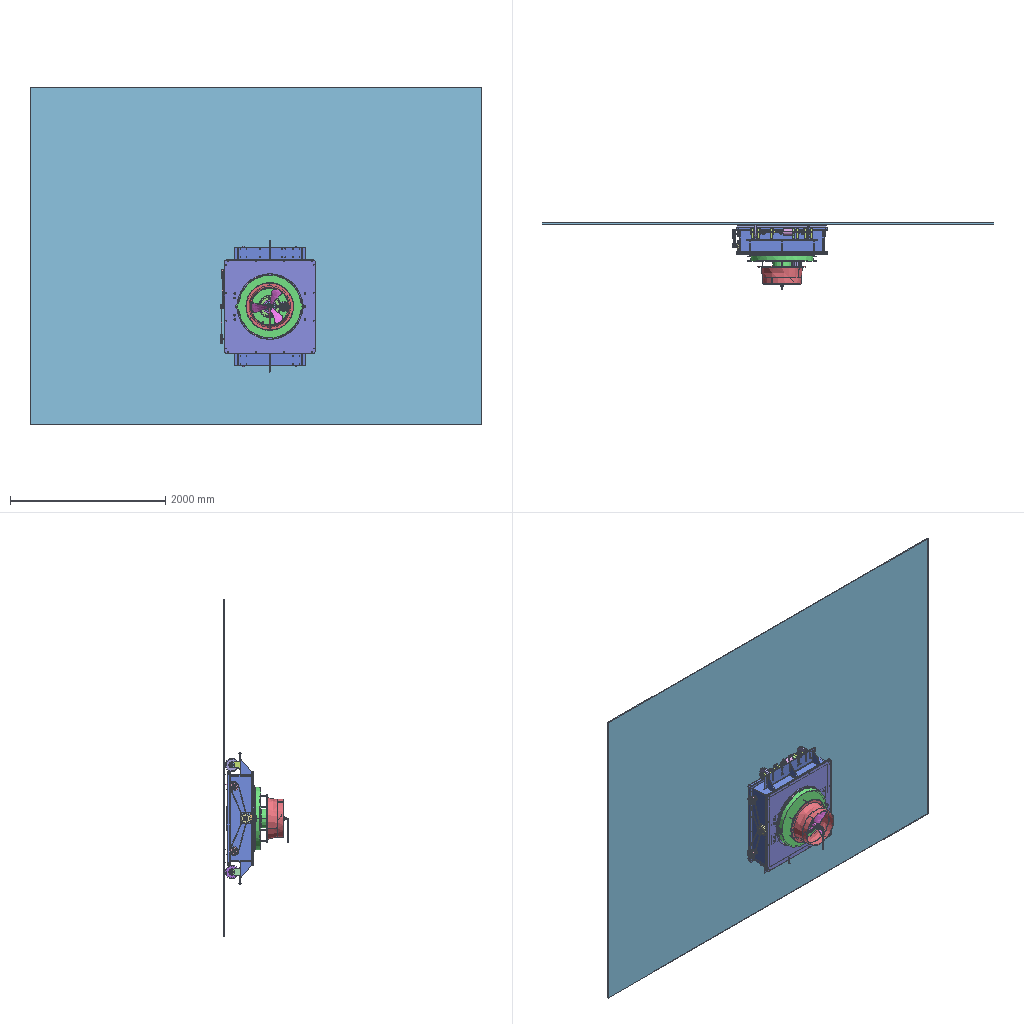Assembly | NX | 147 different items | 274 placed | box 5813 x 845 x 4340 mm
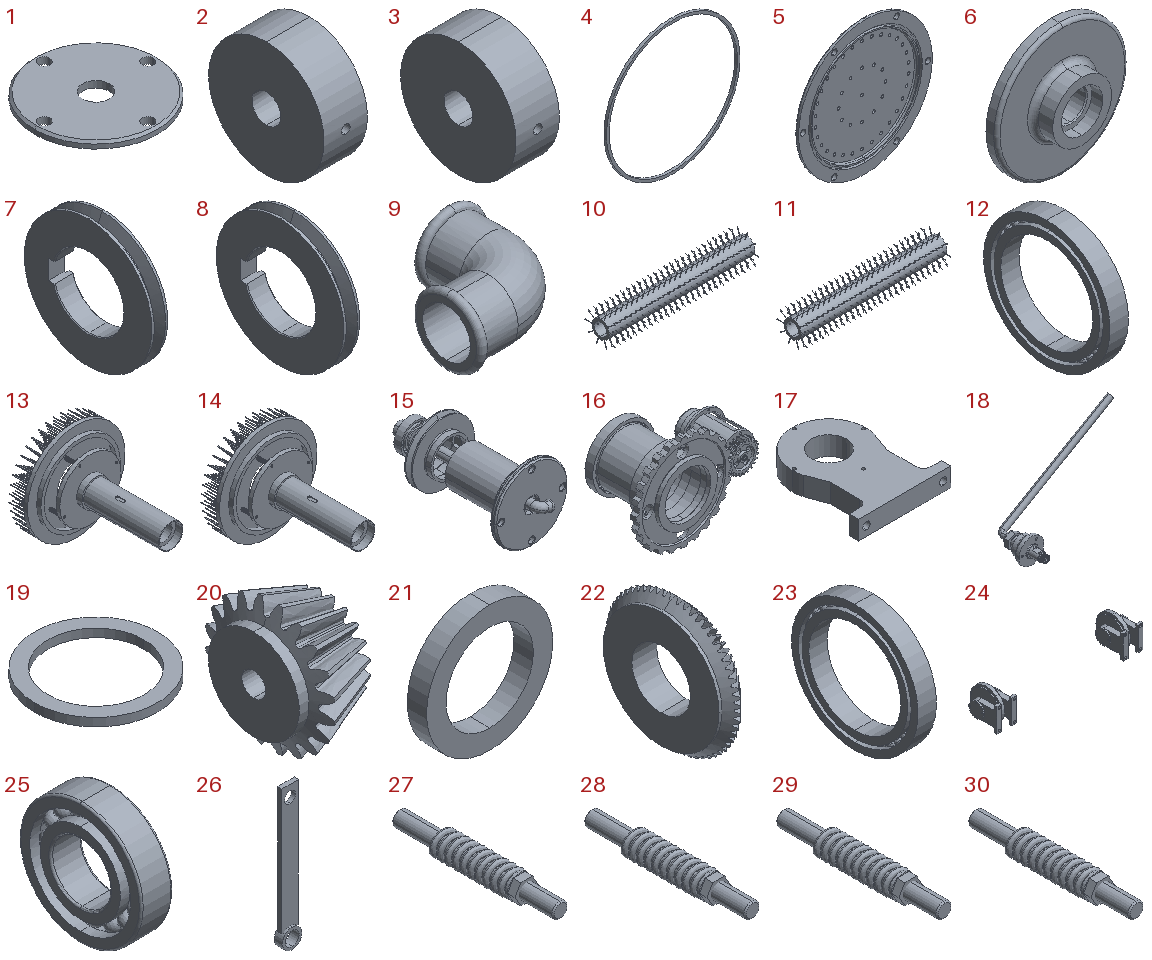Parts list (item | quantity | parent item | size | volume | features):
1 | x2 | in 41 | 171 x 171 x 17 mm | 205475 mm3 | features BREP 1
2 | x2 | in 40 | 30 x 80 x 80 mm | 139671 mm3 | features BREP 1
3 | x2 | in 43 | 30 x 80 x 80 mm | 139671 mm3 | features BREP 1
4 | x2 | in 13, 14 | 102 x 2 x 102 mm | 1257 mm3 | features BREP 1
5 | x2 | in 13, 14 | 120 x 6 x 120 mm | 34469 mm3 | features BREP 1
6 | x2 | in 13, 14 | 120 x 27.99 x 120 mm | 131699 mm3 | features BREP 1
7 | x1 | in 15 | 22 x 145.5 x 145.5 mm | 167430 mm3 | features BREP 1
8 | x1 | in 41 | 22 x 145.5 x 145.5 mm | 167430 mm3 | features BREP 1
9 | x1 | in 41 | 37.5 x 37.5 x 23 mm | 5771 mm3 | features BREP 1
10 | x1 | in 40 | 940 x 212 x 202.242 mm | 4576402 mm3 | features BREP 270
11 | x1 | in 43 | 940 x 212 x 202.242 mm | 4576402 mm3 | features BREP 270
12 | x1 | in 15 | 16 x 110 x 110 mm | 58139 mm3 | features BREP 35
13 | x1 | in 54 | 320 x 372 x 320 mm | 2233372 mm3 | features BREP 11
14 | x1 | in 54 | 320 x 372 x 320 mm | 2233371 mm3 | features BREP 11
15 | x1 | in 54 | 171 x 340.5 x 171 mm | 1447890 mm3 | features BREP 64
16 | x1 | in 54 | 395 x 220 x 292 mm | 2964595 mm3 | features BREP 44
17 | x1 | in 39 | 128 x 156 x 26 mm | 302066 mm3 | features BREP 1
18 | x1 | in 38 | 298.662 x 119 x 190.815 mm | 92954 mm3 | features BREP 3
19 | x1 | in 16 | 180 x 180 x 12 mm | 120637 mm3 | features BREP 1
20 | x1 | in 54 | 36.475 x 65.156 x 65.156 mm | 64691 mm3 | features BREP 1
21 | x2 | in 16 | 13 x 2 x 13 mm | 138.23 mm3 | features BREP 1
22 | x1 | in 54 | 37.656 x 184.108 x 184.108 mm | 545494 mm3 | features BREP 1
23 | x1 | in 41 | 16 x 110 x 110 mm | 58139 mm3 | features BREP 35
24 | x1 | in 54 | 798 x 189 x 168 mm | 2458885 mm3 | features BREP 19
25 | x2 | in 38 | 16 x 62 x 62 mm | 27245 mm3 | features BREP 1
26 | x2 | in 36, 37 | 14 x 6 x 102 mm | 3501 mm3 | features BREP 1
27 | x1 | in 14 | 10 x 64 x 10 mm | 2730 mm3 | features BREP 4
28 | x1 | in 13 | 10 x 64 x 10 mm | 2730 mm3 | features BREP 4
29 | x1 | in 14 | 10 x 64 x 10 mm | 2730 mm3 | features BREP 4
30 | x1 | in 13 | 10 x 64 x 10 mm | 2730 mm3 | features BREP 4
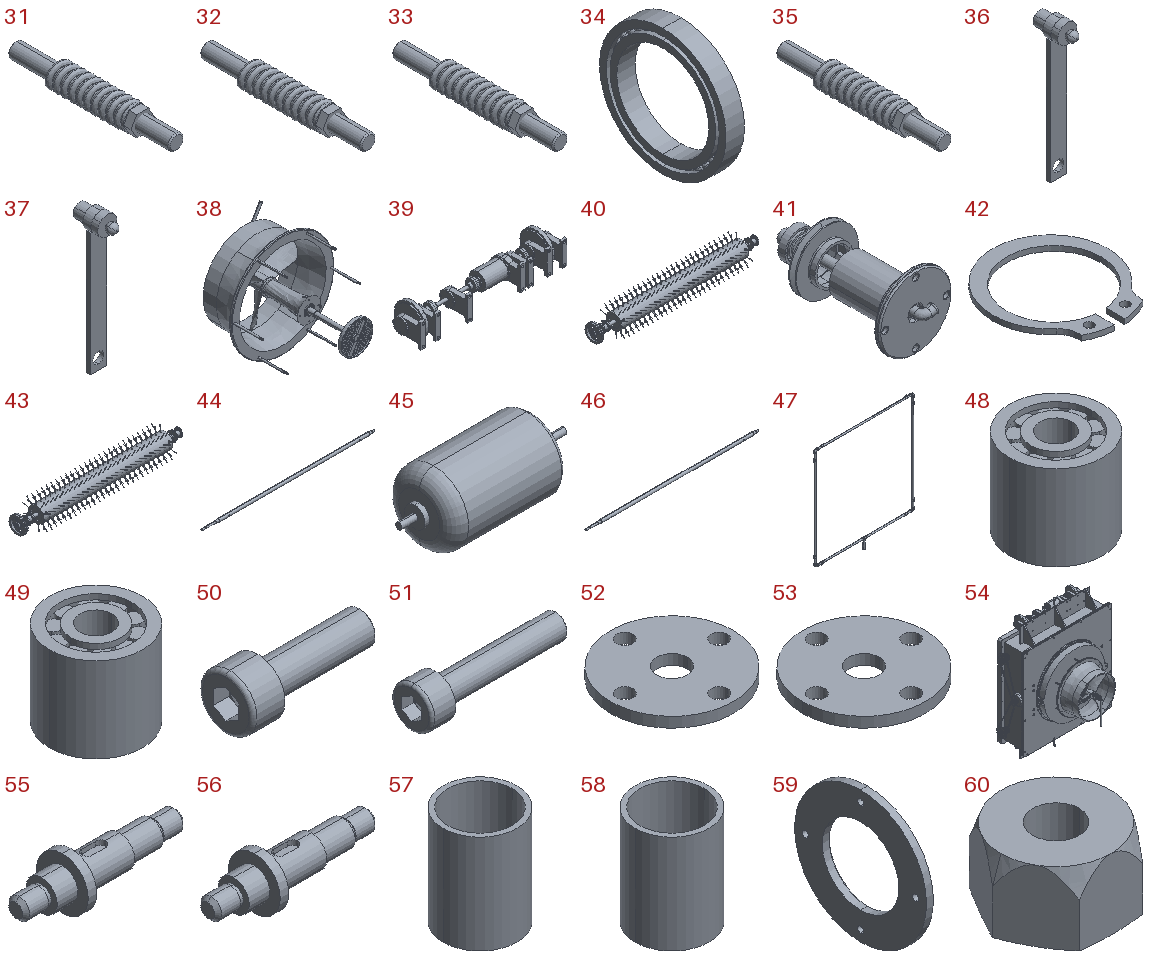31 | x1 | in 13 | 10 x 64 x 10 mm | 2730 mm3 | features BREP 4
32 | x1 | in 14 | 10 x 64 x 10 mm | 2730 mm3 | features BREP 4
33 | x1 | in 13 | 10 x 64 x 10 mm | 2730 mm3 | features BREP 4
34 | x2 | in 54 | 16 x 110 x 110 mm | 58139 mm3 | features BREP 35
35 | x1 | in 14 | 10 x 64 x 10 mm | 2730 mm3 | features BREP 4
36 | x1 | in 54 | 14 x 27.097 x 102 mm | 5636 mm3 | features BREP 3
37 | x1 | in 54 | 14 x 27.097 x 102 mm | 5636 mm3 | features BREP 3
38 | x1 | in 54 | 615 x 737 x 615 mm | 7539199 mm3 | features BREP 16
39 | x1 | in 54 | 798 x 189 x 168 mm | 4416361 mm3 | features BREP 27
40 | x1 | in 54 | 1198 x 209.075 x 210.255 mm | 5412337 mm3 | features BREP 291
41 | x1 | in 54 | 171 x 340.5 x 171 mm | 1447890 mm3 | features BREP 64
42 | x1 | in 38 | 27.2 x 29.93 x 1.2 mm | 263.5 mm3 | features BREP 1
43 | x1 | in 54 | 1184 x 209.075 x 210.255 mm | 5410753 mm3 | features BREP 291
44 | x1 | in 40 | 1181 x 20 x 20 mm | 340275 mm3 | features BREP 1
45 | x1 | in 54 | 321 x 136 x 136 mm | 3154531 mm3 | features BREP 1
46 | x1 | in 43 | 1167 x 20 x 20 mm | 338692 mm3 | features BREP 1
47 | x1 | in 54 | 1091 x 23 x 1199 mm | 156869 mm3 | features BREP 5
48 | x2 | in 40 | 35 x 35 x 32 mm | 21762 mm3 | features BREP 12
49 | x2 | in 43 | 35 x 35 x 32 mm | 21762 mm3 | features BREP 12
50 | x6 | in 38 | 21 x 8.5 x 8.5 mm | 555.936 mm3 | features BREP 1
51 | x1 | in 38 | 30 x 8.5 x 8.5 mm | 732.65 mm3 | features BREP 1
52 | x4 | in 40 | 60 x 60 x 5 mm | 12248 mm3 | features BREP 1
53 | x4 | in 43 | 60 x 60 x 5 mm | 12248 mm3 | features BREP 1
54 | x1 | - | - | 106230951 mm3 | features BREP 907
55 | x2 | in 39 | 93 x 30 x 30 mm | 19864 mm3 | features BREP 1
56 | x2 | in 24 | 93 x 30 x 30 mm | 19864 mm3 | features BREP 1
57 | x2 | in 15 | 92 x 92 x 123 mm | 199391 mm3 | features BREP 1
58 | x2 | in 41 | 92 x 92 x 123 mm | 199391 mm3 | features BREP 1
59 | x2 | in 54 | 11 x 172 x 172 mm | 139981 mm3 | features BREP 1
60 | x1 | in 38 | 9.238 x 8 x 5.3 mm | 239.283 mm3 | features BREP 1
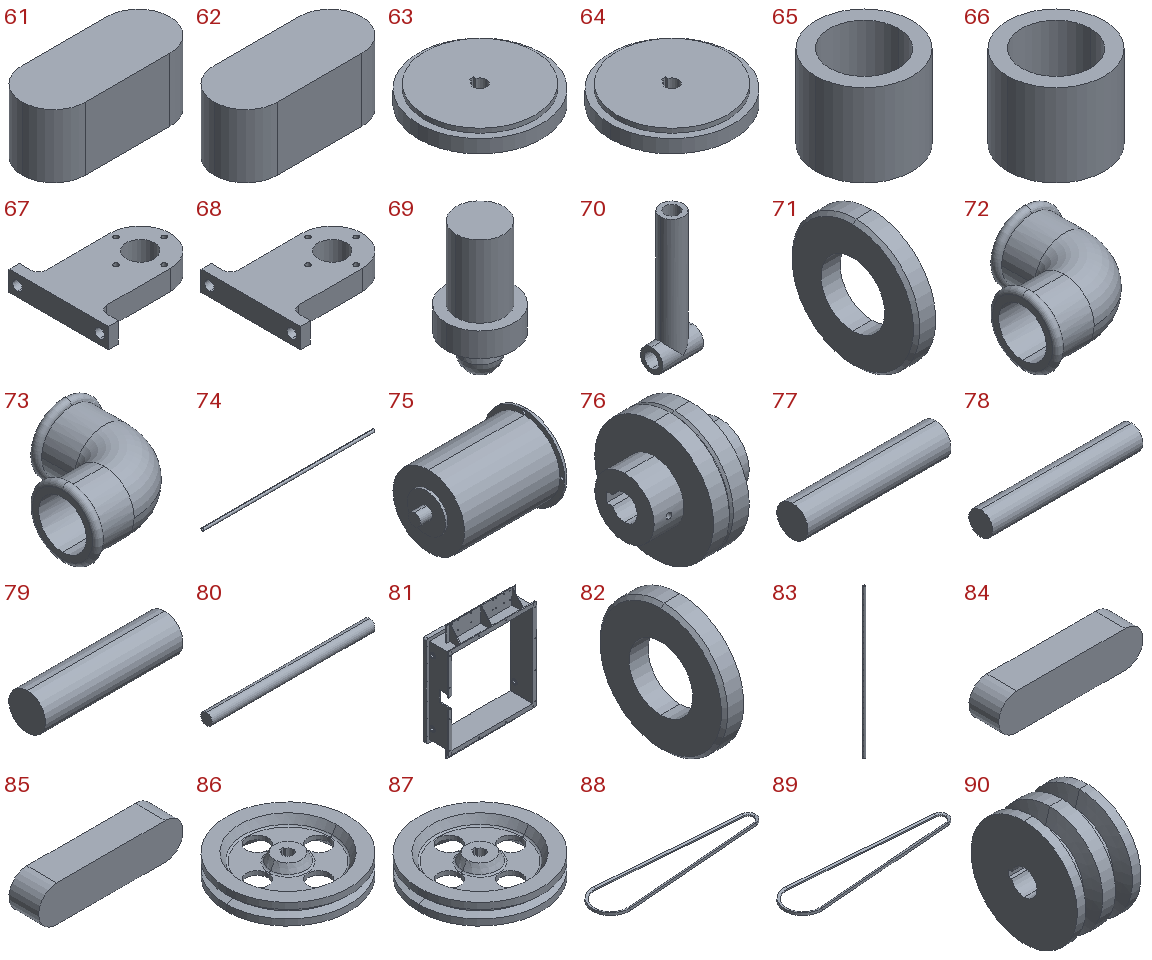61 | x2 | in 39 | 14 x 6 x 6 mm | 457.646 mm3 | features BREP 1
62 | x2 | in 24 | 14 x 6 x 6 mm | 457.646 mm3 | features BREP 1
63 | x2 | in 39 | 168 x 168 x 30 mm | 602860 mm3 | features BREP 1
64 | x2 | in 24 | 168 x 168 x 30 mm | 602860 mm3 | features BREP 1
65 | x2 | in 39 | 21 x 21 x 18 mm | 3054 mm3 | features BREP 1
66 | x2 | in 24 | 21 x 21 x 18 mm | 3054 mm3 | features BREP 1
67 | x6 | in 39 | 144 x 128 x 26 mm | 260725 mm3 | features BREP 1
68 | x4 | in 24 | 144 x 128 x 26 mm | 260725 mm3 | features BREP 1
69 | x2 | in 36, 37 | 14 x 14 x 27.097 mm | 2135 mm3 | features BREP 2
70 | x1 | in 47 | 34 x 19 x 109.5 mm | 21127 mm3 | features BREP 1
71 | x1 | in 40 | 3 x 20 x 20 mm | 699.135 mm3 | features BREP 1
72 | x1 | in 15 | 37.5 x 37.5 x 23 mm | 5771 mm3 | features BREP 1
73 | x4 | in 47 | 37.5 x 37.5 x 23 mm | 5771 mm3 | features BREP 1
74 | x2 | in 47 | 1055 x 16 x 16 mm | 25686 mm3 | features BREP 1
75 | x1 | in 39 | 162 x 102 x 102 mm | 806982 mm3 | features BREP 1
76 | x3 | in 39 | 48 x 60 x 60 mm | 63736 mm3 | features BREP 1
77 | x1 | in 39 | 55 x 12 x 12 mm | 6220 mm3 | features BREP 1
78 | x1 | in 39 | 95 x 15 x 15 mm | 16788 mm3 | features BREP 1
79 | x1 | in 39 | 45 x 12 x 12 mm | 5089 mm3 | features BREP 1
80 | x1 | in 39 | 216 x 15 x 15 mm | 38170 mm3 | features BREP 1
81 | x1 | in 54 | 1170 x 328 x 1520 mm | 26616083 mm3 | features BREP 1
82 | x1 | in 43 | 3 x 20 x 20 mm | 699.135 mm3 | features BREP 1
83 | x2 | in 47 | 16 x 16 x 1015 mm | 24516 mm3 | features BREP 1
84 | x1 | in 40 | 16 x 3.3 x 4 mm | 199.869 mm3 | features BREP 1
85 | x1 | in 43 | 16 x 3.3 x 4 mm | 199.869 mm3 | features BREP 1
86 | x1 | in 40 | 120 x 120 x 20 mm | 115152 mm3 | features BREP 1
87 | x1 | in 43 | 120 x 120 x 20 mm | 115152 mm3 | features BREP 1
88 | x1 | in 54 | 536.48 x 119.96 x 8 mm | 48431 mm3 | features BREP 1
89 | x1 | in 54 | 535.87 x 119.96 x 8 mm | 48380 mm3 | features BREP 1
90 | x1 | in 54 | 30 x 50 x 50 mm | 43819 mm3 | features BREP 1
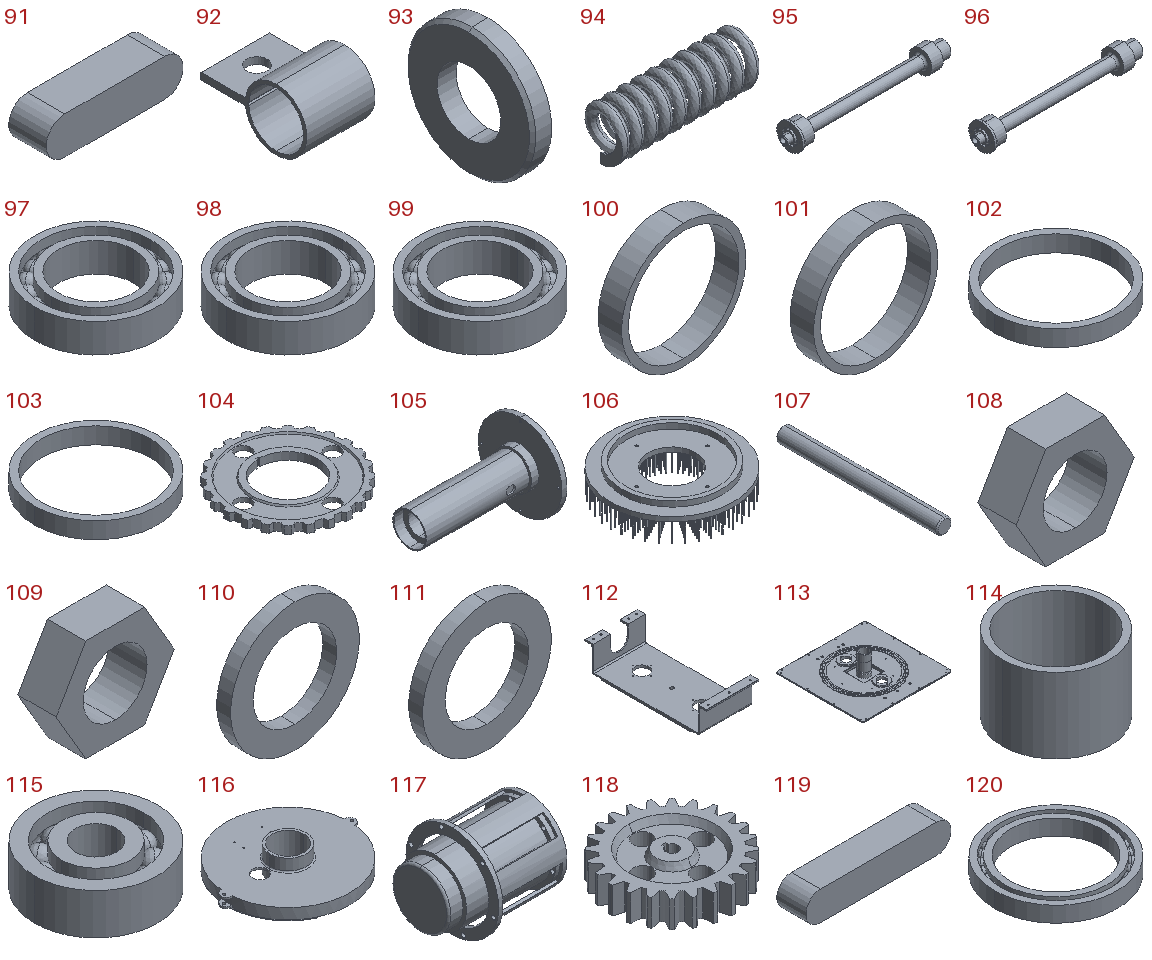91 | x2 | in 54 | 11 x 3 x 3 mm | 93.206 mm3 | features BREP 1
92 | x8 | in 47 | 20 x 31 x 18 mm | 1532 mm3 | features BREP 1
93 | x1 | in 54 | 3 x 20 x 20 mm | 699.135 mm3 | features BREP 1
94 | x8 | in 27, 28, 29, 30, 31, 32, 33, 35 | 30 x 10 x 10 mm | 778.892 mm3 | features BREP 1
95 | x2 | in 15 | 311 x 50 x 50 mm | 154727 mm3 | features BREP 1
96 | x2 | in 41 | 311 x 50 x 50 mm | 154727 mm3 | features BREP 1
97 | x2 | in 15 | 72 x 72 x 17 mm | 29322 mm3 | features BREP 22
98 | x2 | in 41 | 72 x 72 x 17 mm | 29322 mm3 | features BREP 22
99 | x1 | in 54 | 72 x 72 x 17 mm | 29322 mm3 | features BREP 22
100 | x1 | in 15 | 90 x 17 x 90 mm | 22698 mm3 | features BREP 1
101 | x1 | in 41 | 90 x 17 x 90 mm | 22698 mm3 | features BREP 1
102 | x1 | in 15 | 90 x 90 x 12 mm | 16022 mm3 | features BREP 1
103 | x1 | in 41 | 90 x 90 x 12 mm | 16022 mm3 | features BREP 1
104 | x1 | in 16 | 292 x 292 x 18 mm | 597492 mm3 | features BREP 1
105 | x2 | in 13, 14 | 276 x 200 x 200 mm | 1052758 mm3 | features BREP 1
106 | x2 | in 13, 14 | 320 x 320 x 76 mm | 1002124 mm3 | features BREP 1
107 | x8 | in 27, 28, 29, 30, 31, 32, 33, 35 | 6 x 64 x 6 mm | 1805 mm3 | features BREP 1
108 | x2 | in 13, 14 | 9.238 x 3 x 8 mm | 107.372 mm3 | features BREP 1
109 | x8 | in 27, 28, 29, 30, 31, 32, 33, 35 | 9.238 x 3 x 8 mm | 107.372 mm3 | features BREP 1
110 | x2 | in 13, 14 | 9.238 x 1 x 9.238 mm | 38.746 mm3 | features BREP 1
111 | x8 | in 27, 28, 29, 30, 31, 32, 33, 35 | 9.238 x 1 x 9.238 mm | 38.746 mm3 | features BREP 1
112 | x1 | in 54 | 416 x 972 x 217 mm | 7985494 mm3 | features BREP 1
113 | x1 | in 54 | 1200 x 1170 x 281 mm | 20192903 mm3 | features BREP 1
114 | x1 | in 16 | 160 x 160 x 112 mm | 527788 mm3 | features BREP 1
115 | x5 | in 39 | 36 x 36 x 12 mm | 8015 mm3 | features BREP 13
116 | x1 | in 54 | 880 x 808 x 160 mm | 9751568 mm3 | features BREP 1
117 | x1 | in 16 | 176 x 130 x 130 mm | 1047266 mm3 | features BREP 1
118 | x1 | in 16 | 92 x 92 x 20 mm | 80350 mm3 | features BREP 1
119 | x1 | in 16 | 15 x 3 x 3 mm | 129.206 mm3 | features BREP 1
120 | x2 | in 16 | 190 x 190 x 24 mm | 228051 mm3 | features BREP 35
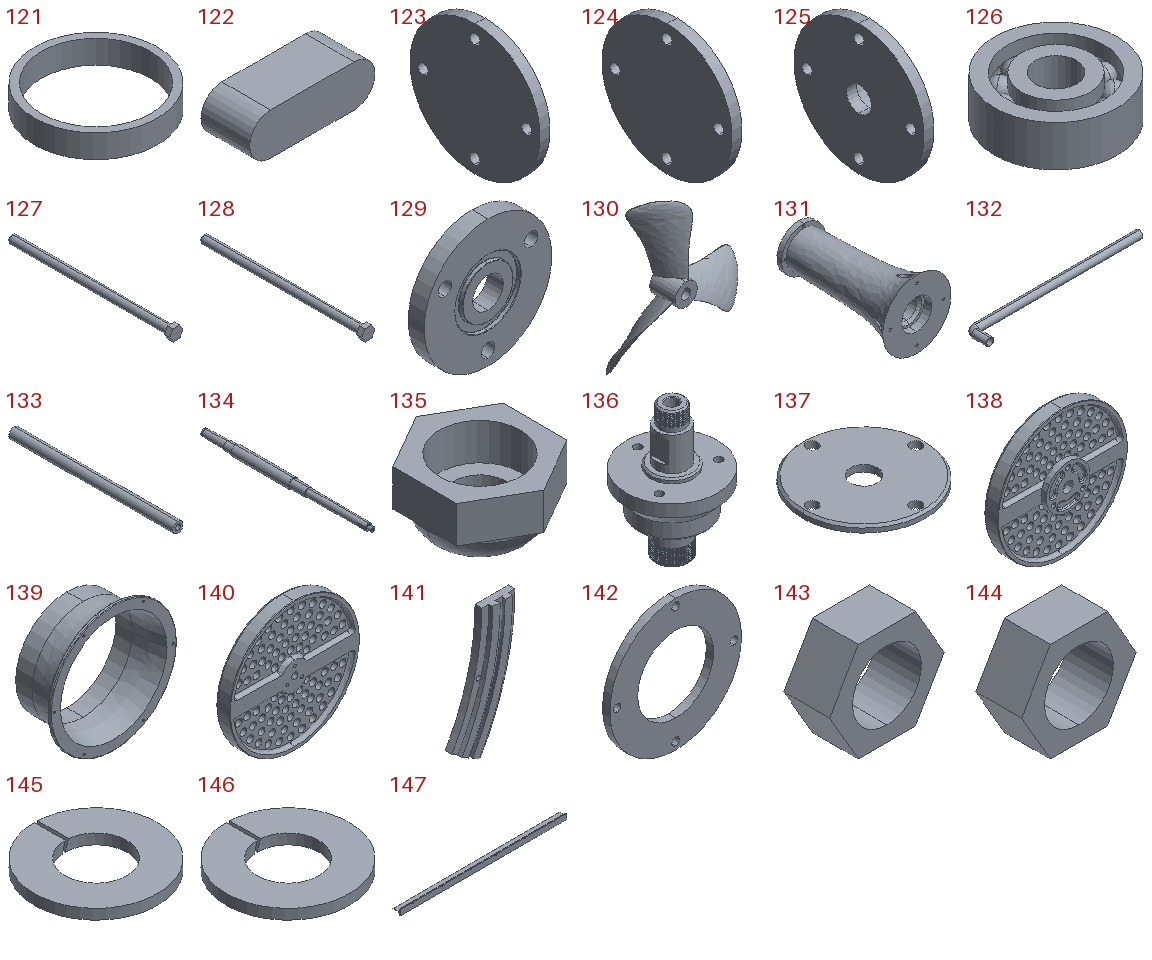121 | x1 | in 16 | 159 x 159 x 30 mm | 133855 mm3 | features BREP 1
122 | x1 | in 16 | 18 x 7 x 6 mm | 701.92 mm3 | features BREP 1
123 | x2 | in 39 | 17 x 78 x 78 mm | 32864 mm3 | features BREP 1
124 | x4 | in 24 | 17 x 78 x 78 mm | 32864 mm3 | features BREP 1
125 | x4 | in 39 | 17 x 78 x 78 mm | 31804 mm3 | features BREP 1
126 | x4 | in 24 | 36 x 36 x 12 mm | 8015 mm3 | features BREP 13
127 | x2 | in 40 | 10 x 124 x 8.66 mm | 3644 mm3 | features BREP 1
128 | x2 | in 43 | 10 x 124 x 8.66 mm | 3644 mm3 | features BREP 1
129 | x1 | in 138 | 64 x 8 x 64 mm | 20301 mm3 | features BREP 1
130 | x1 | in 38 | 443.196 x 101.773 x 427.156 mm | 901902 mm3 | features BREP 1
131 | x1 | in 38 | 140 x 242 x 140 mm | 1087762 mm3 | features BREP 1
132 | x1 | in 18 | 314 x 41 x 14 mm | 13804 mm3 | features BREP 1
133 | x6 | in 38 | 10 x 160 x 10 mm | 9425 mm3 | features BREP 1
134 | x1 | in 38 | 36 x 618 x 36 mm | 396919 mm3 | features BREP 1
135 | x1 | in 18 | 30 x 34.641 x 18 mm | 6874 mm3 | features BREP 1
136 | x1 | in 18 | 60 x 60 x 87 mm | 72276 mm3 | features BREP 1
137 | x2 | in 15 | 171 x 171 x 17 mm | 205475 mm3 | features BREP 1
138 | x1 | in 38 | 190 x 28 x 190 mm | 281154 mm3 | features BREP 2
139 | x1 | in 38 | 615 x 228.661 x 615 mm | 4640014 mm3 | features BREP 1
140 | x1 | in 138 | 190 x 20 x 190 mm | 260933 mm3 | features BREP 1
141 | x6 | in 54 | 102.901 x 18 x 209.5 mm | 150982 mm3 | features BREP 1
142 | x1 | in 38 | 90 x 5 x 90 mm | 20765 mm3 | features BREP 1
143 | x2 | in 40 | 10 x 4 x 8.66 mm | 146.71 mm3 | features BREP 1
144 | x2 | in 43 | 10 x 4 x 8.66 mm | 146.71 mm3 | features BREP 1
145 | x2 | in 40 | 12 x 12 x 1 mm | 83.879 mm3 | features BREP 1
146 | x2 | in 43 | 12 x 12 x 1 mm | 83.879 mm3 | features BREP 1
147 | x2 | in 54 | 1146 x 50 x 39 mm | 357645 mm3 | features BREP 1